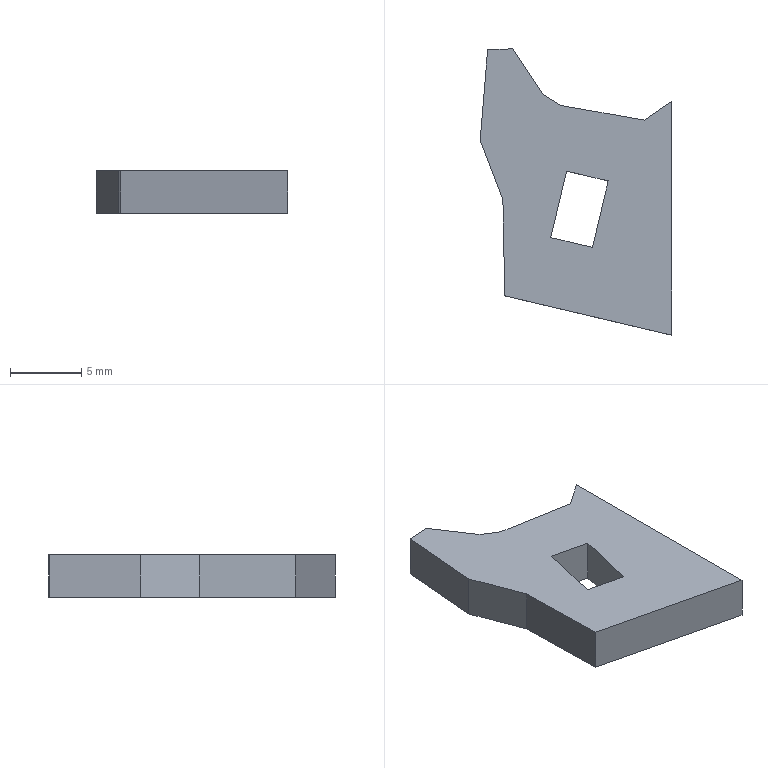Part | SolidWorks | features BaseBody 1 | 1 solid | 16 faces | box 13.422 x 20.055 x 3 mm | volume 525.703 mm3 | spline 9 | plane 7
STEP:
#1=CARTESIAN_POINT('',(-7.64,4.495,-1.5));
#2=VERTEX_POINT('',#1);
#3=CARTESIAN_POINT('',(-8.743,-0.1604,-1.5));
#4=VERTEX_POINT('',#3);
#5=CARTESIAN_POINT('',(-8.242,1.953,-1.5));
#6=DIRECTION('',(-0.2306,-0.9731,0.));
#7=VECTOR('',#6,1000.);
#8=LINE('',#5,#7);
#9=EDGE_CURVE('',#2,#4,#8,.T.);
#10=ORIENTED_EDGE('',*,*,#9,.F.);
#11=CARTESIAN_POINT('',(-7.64,4.495,1.5));
#12=VERTEX_POINT('',#11);
#13=CARTESIAN_POINT('',(-7.64,4.495,1.5));
#14=DIRECTION('',(0.,0.,-1.));
#15=VECTOR('',#14,1000.);
#16=LINE('',#13,#15);
#17=EDGE_CURVE('',#12,#2,#16,.T.);
#18=ORIENTED_EDGE('',*,*,#17,.F.);
#19=CARTESIAN_POINT('',(-8.743,-0.1604,1.5));
#20=VERTEX_POINT('',#19);
#21=CARTESIAN_POINT('',(-8.242,1.953,1.5));
#22=DIRECTION('',(-0.2306,-0.9731,0.));
#23=VECTOR('',#22,1000.);
#24=LINE('',#21,#23);
#25=EDGE_CURVE('',#12,#20,#24,.T.);
#26=ORIENTED_EDGE('',*,*,#25,.T.);
#27=CARTESIAN_POINT('',(-8.743,-0.1604,1.5));
#28=DIRECTION('',(0.,0.,-1.));
#29=VECTOR('',#28,1000.);
#30=LINE('',#27,#29);
#31=EDGE_CURVE('',#20,#4,#30,.T.);
#32=ORIENTED_EDGE('',*,*,#31,.T.);
#33=EDGE_LOOP('',(#10,#18,#26,#32));
#34=FACE_OUTER_BOUND('',#33,.T.);
#35=CARTESIAN_POINT('',(-8.242,1.953,1.5));
#36=DIRECTION('',(0.9731,-0.2306,0.));
#37=DIRECTION('',(0.,0.,-1.));
#38=AXIS2_PLACEMENT_3D('',#35,#36,#37);
#39=PLANE('',#38);
#40=ADVANCED_FACE('',(#34),#39,.T.);
#41=CARTESIAN_POINT('',(-4.721,3.803,-1.5));
#42=VERTEX_POINT('',#41);
#43=CARTESIAN_POINT('',(0.6024,2.542,-1.5));
#44=DIRECTION('',(-0.9731,0.2306,0.));
#45=VECTOR('',#44,1000.);
#46=LINE('',#43,#45);
#47=EDGE_CURVE('',#42,#2,#46,.T.);
#48=ORIENTED_EDGE('',*,*,#47,.F.);
#49=CARTESIAN_POINT('',(-4.721,3.803,1.5));
#50=VERTEX_POINT('',#49);
#51=CARTESIAN_POINT('',(-4.721,3.803,1.5));
#52=DIRECTION('',(0.,0.,-1.));
#53=VECTOR('',#52,1000.);
#54=LINE('',#51,#53);
#55=EDGE_CURVE('',#50,#42,#54,.T.);
#56=ORIENTED_EDGE('',*,*,#55,.F.);
#57=CARTESIAN_POINT('',(0.6024,2.542,1.5));
#58=DIRECTION('',(-0.9731,0.2306,0.));
#59=VECTOR('',#58,1000.);
#60=LINE('',#57,#59);
#61=EDGE_CURVE('',#50,#12,#60,.T.);
#62=ORIENTED_EDGE('',*,*,#61,.T.);
#63=ORIENTED_EDGE('',*,*,#17,.T.);
#64=EDGE_LOOP('',(#48,#56,#62,#63));
#65=FACE_OUTER_BOUND('',#64,.T.);
#66=CARTESIAN_POINT('',(0.6024,2.542,1.5));
#67=DIRECTION('',(-0.2306,-0.9731,0.));
#68=DIRECTION('',(-0.9731,0.2306,0.));
#69=AXIS2_PLACEMENT_3D('',#66,#67,#68);
#70=PLANE('',#69);
#71=ADVANCED_FACE('',(#65),#70,.T.);
#72=CARTESIAN_POINT('',(-5.824,-0.8521,-1.5));
#73=VERTEX_POINT('',#72);
#74=CARTESIAN_POINT('',(-5.323,1.261,-1.5));
#75=DIRECTION('',(-0.2306,-0.9731,0.));
#76=VECTOR('',#75,1000.);
#77=LINE('',#74,#76);
#78=EDGE_CURVE('',#42,#73,#77,.T.);
#79=ORIENTED_EDGE('',*,*,#78,.T.);
#80=CARTESIAN_POINT('',(-5.824,-0.8521,1.5));
#81=VERTEX_POINT('',#80);
#82=CARTESIAN_POINT('',(-5.824,-0.8521,1.5));
#83=DIRECTION('',(0.,0.,-1.));
#84=VECTOR('',#83,1000.);
#85=LINE('',#82,#84);
#86=EDGE_CURVE('',#81,#73,#85,.T.);
#87=ORIENTED_EDGE('',*,*,#86,.F.);
#88=CARTESIAN_POINT('',(-5.323,1.261,1.5));
#89=DIRECTION('',(-0.2306,-0.9731,0.));
#90=VECTOR('',#89,1000.);
#91=LINE('',#88,#90);
#92=EDGE_CURVE('',#50,#81,#91,.T.);
#93=ORIENTED_EDGE('',*,*,#92,.F.);
#94=ORIENTED_EDGE('',*,*,#55,.T.);
#95=EDGE_LOOP('',(#79,#87,#93,#94));
#96=FACE_OUTER_BOUND('',#95,.T.);
#97=CARTESIAN_POINT('',(-5.323,1.261,1.5));
#98=DIRECTION('',(0.9731,-0.2306,0.));
#99=DIRECTION('',(0.,0.,-1.));
#100=AXIS2_PLACEMENT_3D('',#97,#98,#99);
#101=PLANE('',#100);
#102=ADVANCED_FACE('',(#96),#101,.F.);
#103=CARTESIAN_POINT('',(-0.5008,-2.113,-1.5));
#104=DIRECTION('',(-0.9731,0.2306,0.));
#105=VECTOR('',#104,1000.);
#106=LINE('',#103,#105);
#107=EDGE_CURVE('',#73,#4,#106,.T.);
#108=ORIENTED_EDGE('',*,*,#107,.T.);
#109=ORIENTED_EDGE('',*,*,#31,.F.);
#110=CARTESIAN_POINT('',(-0.5008,-2.113,1.5));
#111=DIRECTION('',(-0.9731,0.2306,0.));
#112=VECTOR('',#111,1000.);
#113=LINE('',#110,#112);
#114=EDGE_CURVE('',#81,#20,#113,.T.);
#115=ORIENTED_EDGE('',*,*,#114,.F.);
#116=ORIENTED_EDGE('',*,*,#86,.T.);
#117=EDGE_LOOP('',(#108,#109,#115,#116));
#118=FACE_OUTER_BOUND('',#117,.T.);
#119=CARTESIAN_POINT('',(-0.5008,-2.113,1.5));
#120=DIRECTION('',(-0.2306,-0.9731,0.));
#121=DIRECTION('',(-0.9731,0.2306,0.));
#122=AXIS2_PLACEMENT_3D('',#119,#120,#121);
#123=PLANE('',#122);
#124=ADVANCED_FACE('',(#118),#123,.F.);
#125=ORIENTED_EDGE('',*,*,#9,.T.);
#126=ORIENTED_EDGE('',*,*,#107,.F.);
#127=ORIENTED_EDGE('',*,*,#78,.F.);
#128=ORIENTED_EDGE('',*,*,#47,.T.);
#129=EDGE_LOOP('',(#125,#126,#127,#128));
#130=FACE_BOUND('',#129,.T.);
#131=CARTESIAN_POINT('',(-0.264,9.379,-1.5));
#132=VERTEX_POINT('',#131);
#133=CARTESIAN_POINT('',(-2.191,8.063,-1.5));
#134=VERTEX_POINT('',#133);
#135=CARTESIAN_POINT('',(-0.264,9.379,-1.5));
#136=CARTESIAN_POINT('',(-0.9053,8.941,-1.5));
#137=CARTESIAN_POINT('',(-1.55,8.503,-1.5));
#138=CARTESIAN_POINT('',(-2.191,8.063,-1.5));
#139=B_SPLINE_CURVE_WITH_KNOTS('',3,(#135,#136,#137,#138),.UNSPECIFIED.,.F.,.F.,(4,4),(0.4737,0.5263),.UNSPECIFIED.);
#140=EDGE_CURVE('',#132,#134,#139,.T.);
#141=ORIENTED_EDGE('',*,*,#140,.F.);
#142=CARTESIAN_POINT('',(-0.264,-6.995,-1.5));
#143=VERTEX_POINT('',#142);
#144=CARTESIAN_POINT('',(-0.264,9.379,-1.5));
#145=DIRECTION('',(0.,-1.,0.));
#146=VECTOR('',#145,1000.);
#147=LINE('',#144,#146);
#148=EDGE_CURVE('',#132,#143,#147,.T.);
#149=ORIENTED_EDGE('',*,*,#148,.T.);
#150=CARTESIAN_POINT('',(-11.964,-4.235,-1.5));
#151=VERTEX_POINT('',#150);
#152=CARTESIAN_POINT('',(-11.964,-4.235,-1.5));
#153=CARTESIAN_POINT('',(-8.063,-5.155,-1.5));
#154=CARTESIAN_POINT('',(-4.164,-6.075,-1.5));
#155=CARTESIAN_POINT('',(-0.264,-6.995,-1.5));
#156=B_SPLINE_CURVE_WITH_KNOTS('',3,(#152,#153,#154,#155),.UNSPECIFIED.,.F.,.F.,(4,4),(0.8947,1.),.UNSPECIFIED.);
#157=EDGE_CURVE('',#151,#143,#156,.T.);
#158=ORIENTED_EDGE('',*,*,#157,.F.);
#159=CARTESIAN_POINT('',(-12.094,2.485,-1.5));
#160=VERTEX_POINT('',#159);
#161=CARTESIAN_POINT('',(-12.094,2.485,-1.5));
#162=CARTESIAN_POINT('',(-12.051,0.2468,-1.5));
#163=CARTESIAN_POINT('',(-12.008,-1.995,-1.5));
#164=CARTESIAN_POINT('',(-11.964,-4.235,-1.5));
#165=B_SPLINE_CURVE_WITH_KNOTS('',3,(#161,#162,#163,#164),.UNSPECIFIED.,.F.,.F.,(4,4),(0.8421,0.8947),.UNSPECIFIED.);
#166=EDGE_CURVE('',#160,#151,#165,.T.);
#167=ORIENTED_EDGE('',*,*,#166,.F.);
#168=CARTESIAN_POINT('',(-13.686,6.633,-1.5));
#169=VERTEX_POINT('',#168);
#170=CARTESIAN_POINT('',(-13.686,6.633,-1.5));
#171=CARTESIAN_POINT('',(-13.157,5.251,-1.5));
#172=CARTESIAN_POINT('',(-12.626,3.868,-1.5));
#173=CARTESIAN_POINT('',(-12.094,2.485,-1.5));
#174=B_SPLINE_CURVE_WITH_KNOTS('',3,(#170,#171,#172,#173),.UNSPECIFIED.,.F.,.F.,(4,4),(0.7895,0.8421),.UNSPECIFIED.);
#175=EDGE_CURVE('',#169,#160,#174,.T.);
#176=ORIENTED_EDGE('',*,*,#175,.F.);
#177=CARTESIAN_POINT('',(-13.167,12.98,-1.5));
#178=VERTEX_POINT('',#177);
#179=CARTESIAN_POINT('',(-13.167,12.98,-1.5));
#180=CARTESIAN_POINT('',(-13.338,10.864,-1.5));
#181=CARTESIAN_POINT('',(-13.513,8.749,-1.5));
#182=CARTESIAN_POINT('',(-13.686,6.633,-1.5));
#183=B_SPLINE_CURVE_WITH_KNOTS('',3,(#179,#180,#181,#182),.UNSPECIFIED.,.F.,.F.,(4,4),(0.7368,0.7895),.UNSPECIFIED.);
#184=EDGE_CURVE('',#178,#169,#183,.T.);
#185=ORIENTED_EDGE('',*,*,#184,.F.);
#186=CARTESIAN_POINT('',(-11.425,13.059,-1.5));
#187=VERTEX_POINT('',#186);
#188=CARTESIAN_POINT('',(-11.425,13.059,-1.5));
#189=CARTESIAN_POINT('',(-12.004,13.035,-1.5));
#190=CARTESIAN_POINT('',(-12.584,13.006,-1.5));
#191=CARTESIAN_POINT('',(-13.167,12.98,-1.5));
#192=B_SPLINE_CURVE_WITH_KNOTS('',3,(#188,#189,#190,#191),.UNSPECIFIED.,.F.,.F.,(4,4),(0.6842,0.7368),.UNSPECIFIED.);
#193=EDGE_CURVE('',#187,#178,#192,.T.);
#194=ORIENTED_EDGE('',*,*,#193,.F.);
#195=CARTESIAN_POINT('',(-9.322,9.892,-1.5));
#196=VERTEX_POINT('',#195);
#197=CARTESIAN_POINT('',(-9.322,9.892,-1.5));
#198=CARTESIAN_POINT('',(-10.022,10.947,-1.5));
#199=CARTESIAN_POINT('',(-10.724,12.004,-1.5));
#200=CARTESIAN_POINT('',(-11.425,13.059,-1.5));
#201=B_SPLINE_CURVE_WITH_KNOTS('',3,(#197,#198,#199,#200),.UNSPECIFIED.,.F.,.F.,(4,4),(0.6316,0.6842),.UNSPECIFIED.);
#202=EDGE_CURVE('',#196,#187,#201,.T.);
#203=ORIENTED_EDGE('',*,*,#202,.F.);
#204=CARTESIAN_POINT('',(-8.049,9.09,-1.5));
#205=VERTEX_POINT('',#204);
#206=CARTESIAN_POINT('',(-8.049,9.09,-1.5));
#207=CARTESIAN_POINT('',(-8.471,9.357,-1.5));
#208=CARTESIAN_POINT('',(-8.897,9.624,-1.5));
#209=CARTESIAN_POINT('',(-9.322,9.892,-1.5));
#210=B_SPLINE_CURVE_WITH_KNOTS('',3,(#206,#207,#208,#209),.UNSPECIFIED.,.F.,.F.,(4,4),(0.5789,0.6316),.UNSPECIFIED.);
#211=EDGE_CURVE('',#205,#196,#210,.T.);
#212=ORIENTED_EDGE('',*,*,#211,.F.);
#213=CARTESIAN_POINT('',(-2.191,8.063,-1.5));
#214=CARTESIAN_POINT('',(-4.141,8.406,-1.5));
#215=CARTESIAN_POINT('',(-6.094,8.747,-1.5));
#216=CARTESIAN_POINT('',(-8.049,9.09,-1.5));
#217=B_SPLINE_CURVE_WITH_KNOTS('',3,(#213,#214,#215,#216),.UNSPECIFIED.,.F.,.F.,(4,4),(0.5263,0.5789),.UNSPECIFIED.);
#218=EDGE_CURVE('',#134,#205,#217,.T.);
#219=ORIENTED_EDGE('',*,*,#218,.F.);
#220=EDGE_LOOP('',(#141,#149,#158,#167,#176,#185,#194,#203,#212,#219));
#221=FACE_OUTER_BOUND('',#220,.T.);
#222=CARTESIAN_POINT('',(-1.228,8.722,-1.5));
#223=DIRECTION('',(0.,0.,1.));
#224=DIRECTION('',(1.,0.,0.));
#225=AXIS2_PLACEMENT_3D('',#222,#223,#224);
#226=PLANE('',#225);
#227=ADVANCED_FACE('',(#130,#221),#226,.F.);
#228=ORIENTED_EDGE('',*,*,#114,.T.);
#229=ORIENTED_EDGE('',*,*,#25,.F.);
#230=ORIENTED_EDGE('',*,*,#61,.F.);
#231=ORIENTED_EDGE('',*,*,#92,.T.);
#232=EDGE_LOOP('',(#228,#229,#230,#231));
#233=FACE_BOUND('',#232,.T.);
#234=CARTESIAN_POINT('',(-0.264,9.379,1.5));
#235=VERTEX_POINT('',#234);
#236=CARTESIAN_POINT('',(-2.191,8.063,1.5));
#237=VERTEX_POINT('',#236);
#238=CARTESIAN_POINT('',(-0.264,9.379,1.5));
#239=CARTESIAN_POINT('',(-0.9053,8.941,1.5));
#240=CARTESIAN_POINT('',(-1.55,8.503,1.5));
#241=CARTESIAN_POINT('',(-2.191,8.063,1.5));
#242=B_SPLINE_CURVE_WITH_KNOTS('',3,(#238,#239,#240,#241),.UNSPECIFIED.,.F.,.F.,(4,4),(0.4737,0.5263),.UNSPECIFIED.);
#243=EDGE_CURVE('',#235,#237,#242,.T.);
#244=ORIENTED_EDGE('',*,*,#243,.T.);
#245=CARTESIAN_POINT('',(-8.049,9.09,1.5));
#246=VERTEX_POINT('',#245);
#247=CARTESIAN_POINT('',(-2.191,8.063,1.5));
#248=CARTESIAN_POINT('',(-4.141,8.406,1.5));
#249=CARTESIAN_POINT('',(-6.094,8.747,1.5));
#250=CARTESIAN_POINT('',(-8.049,9.09,1.5));
#251=B_SPLINE_CURVE_WITH_KNOTS('',3,(#247,#248,#249,#250),.UNSPECIFIED.,.F.,.F.,(4,4),(0.5263,0.5789),.UNSPECIFIED.);
#252=EDGE_CURVE('',#237,#246,#251,.T.);
#253=ORIENTED_EDGE('',*,*,#252,.T.);
#254=CARTESIAN_POINT('',(-9.322,9.892,1.5));
#255=VERTEX_POINT('',#254);
#256=CARTESIAN_POINT('',(-8.049,9.09,1.5));
#257=CARTESIAN_POINT('',(-8.471,9.357,1.5));
#258=CARTESIAN_POINT('',(-8.897,9.624,1.5));
#259=CARTESIAN_POINT('',(-9.322,9.892,1.5));
#260=B_SPLINE_CURVE_WITH_KNOTS('',3,(#256,#257,#258,#259),.UNSPECIFIED.,.F.,.F.,(4,4),(0.5789,0.6316),.UNSPECIFIED.);
#261=EDGE_CURVE('',#246,#255,#260,.T.);
#262=ORIENTED_EDGE('',*,*,#261,.T.);
#263=CARTESIAN_POINT('',(-11.425,13.059,1.5));
#264=VERTEX_POINT('',#263);
#265=CARTESIAN_POINT('',(-9.322,9.892,1.5));
#266=CARTESIAN_POINT('',(-10.022,10.947,1.5));
#267=CARTESIAN_POINT('',(-10.724,12.004,1.5));
#268=CARTESIAN_POINT('',(-11.425,13.059,1.5));
#269=B_SPLINE_CURVE_WITH_KNOTS('',3,(#265,#266,#267,#268),.UNSPECIFIED.,.F.,.F.,(4,4),(0.6316,0.6842),.UNSPECIFIED.);
#270=EDGE_CURVE('',#255,#264,#269,.T.);
#271=ORIENTED_EDGE('',*,*,#270,.T.);
#272=CARTESIAN_POINT('',(-13.167,12.98,1.5));
#273=VERTEX_POINT('',#272);
#274=CARTESIAN_POINT('',(-11.425,13.059,1.5));
#275=CARTESIAN_POINT('',(-12.004,13.035,1.5));
#276=CARTESIAN_POINT('',(-12.584,13.006,1.5));
#277=CARTESIAN_POINT('',(-13.167,12.98,1.5));
#278=B_SPLINE_CURVE_WITH_KNOTS('',3,(#274,#275,#276,#277),.UNSPECIFIED.,.F.,.F.,(4,4),(0.6842,0.7368),.UNSPECIFIED.);
#279=EDGE_CURVE('',#264,#273,#278,.T.);
#280=ORIENTED_EDGE('',*,*,#279,.T.);
#281=CARTESIAN_POINT('',(-13.686,6.633,1.5));
#282=VERTEX_POINT('',#281);
#283=CARTESIAN_POINT('',(-13.167,12.98,1.5));
#284=CARTESIAN_POINT('',(-13.338,10.864,1.5));
#285=CARTESIAN_POINT('',(-13.513,8.749,1.5));
#286=CARTESIAN_POINT('',(-13.686,6.633,1.5));
#287=B_SPLINE_CURVE_WITH_KNOTS('',3,(#283,#284,#285,#286),.UNSPECIFIED.,.F.,.F.,(4,4),(0.7368,0.7895),.UNSPECIFIED.);
#288=EDGE_CURVE('',#273,#282,#287,.T.);
#289=ORIENTED_EDGE('',*,*,#288,.T.);
#290=CARTESIAN_POINT('',(-12.094,2.485,1.5));
#291=VERTEX_POINT('',#290);
#292=CARTESIAN_POINT('',(-13.686,6.633,1.5));
#293=CARTESIAN_POINT('',(-13.157,5.251,1.5));
#294=CARTESIAN_POINT('',(-12.626,3.868,1.5));
#295=CARTESIAN_POINT('',(-12.094,2.485,1.5));
#296=B_SPLINE_CURVE_WITH_KNOTS('',3,(#292,#293,#294,#295),.UNSPECIFIED.,.F.,.F.,(4,4),(0.7895,0.8421),.UNSPECIFIED.);
#297=EDGE_CURVE('',#282,#291,#296,.T.);
#298=ORIENTED_EDGE('',*,*,#297,.T.);
#299=CARTESIAN_POINT('',(-11.964,-4.235,1.5));
#300=VERTEX_POINT('',#299);
#301=CARTESIAN_POINT('',(-12.094,2.485,1.5));
#302=CARTESIAN_POINT('',(-12.051,0.2468,1.5));
#303=CARTESIAN_POINT('',(-12.008,-1.995,1.5));
#304=CARTESIAN_POINT('',(-11.964,-4.235,1.5));
#305=B_SPLINE_CURVE_WITH_KNOTS('',3,(#301,#302,#303,#304),.UNSPECIFIED.,.F.,.F.,(4,4),(0.8421,0.8947),.UNSPECIFIED.);
#306=EDGE_CURVE('',#291,#300,#305,.T.);
#307=ORIENTED_EDGE('',*,*,#306,.T.);
#308=CARTESIAN_POINT('',(-0.264,-6.995,1.5));
#309=VERTEX_POINT('',#308);
#310=CARTESIAN_POINT('',(-11.964,-4.235,1.5));
#311=CARTESIAN_POINT('',(-8.063,-5.155,1.5));
#312=CARTESIAN_POINT('',(-4.164,-6.075,1.5));
#313=CARTESIAN_POINT('',(-0.264,-6.995,1.5));
#314=B_SPLINE_CURVE_WITH_KNOTS('',3,(#310,#311,#312,#313),.UNSPECIFIED.,.F.,.F.,(4,4),(0.8947,1.),.UNSPECIFIED.);
#315=EDGE_CURVE('',#300,#309,#314,.T.);
#316=ORIENTED_EDGE('',*,*,#315,.T.);
#317=CARTESIAN_POINT('',(-0.264,9.379,1.5));
#318=DIRECTION('',(0.,-1.,0.));
#319=VECTOR('',#318,1000.);
#320=LINE('',#317,#319);
#321=EDGE_CURVE('',#235,#309,#320,.T.);
#322=ORIENTED_EDGE('',*,*,#321,.F.);
#323=EDGE_LOOP('',(#244,#253,#262,#271,#280,#289,#298,#307,#316,#322));
#324=FACE_OUTER_BOUND('',#323,.T.);
#325=CARTESIAN_POINT('',(-1.228,8.722,1.5));
#326=DIRECTION('',(0.,0.,1.));
#327=DIRECTION('',(1.,0.,0.));
#328=AXIS2_PLACEMENT_3D('',#325,#326,#327);
#329=PLANE('',#328);
#330=ADVANCED_FACE('',(#233,#324),#329,.T.);
#331=ORIENTED_EDGE('',*,*,#148,.F.);
#332=CARTESIAN_POINT('',(-0.264,9.379,1.5));
#333=DIRECTION('',(0.,0.,-1.));
#334=VECTOR('',#333,1000.);
#335=LINE('',#332,#334);
#336=EDGE_CURVE('',#235,#132,#335,.T.);
#337=ORIENTED_EDGE('',*,*,#336,.F.);
#338=ORIENTED_EDGE('',*,*,#321,.T.);
#339=CARTESIAN_POINT('',(-0.264,-6.995,1.5));
#340=DIRECTION('',(0.,0.,-1.));
#341=VECTOR('',#340,1000.);
#342=LINE('',#339,#341);
#343=EDGE_CURVE('',#309,#143,#342,.T.);
#344=ORIENTED_EDGE('',*,*,#343,.T.);
#345=EDGE_LOOP('',(#331,#337,#338,#344));
#346=FACE_OUTER_BOUND('',#345,.T.);
#347=CARTESIAN_POINT('',(-0.264,9.379,1.5));
#348=DIRECTION('',(1.,0.,0.));
#349=DIRECTION('',(0.,1.,0.));
#350=AXIS2_PLACEMENT_3D('',#347,#348,#349);
#351=PLANE('',#350);
#352=ADVANCED_FACE('',(#346),#351,.T.);
#353=ORIENTED_EDGE('',*,*,#157,.T.);
#354=ORIENTED_EDGE('',*,*,#343,.F.);
#355=ORIENTED_EDGE('',*,*,#315,.F.);
#356=CARTESIAN_POINT('',(-11.964,-4.235,1.5));
#357=DIRECTION('',(0.,0.,-1.));
#358=VECTOR('',#357,1000.);
#359=LINE('',#356,#358);
#360=EDGE_CURVE('',#300,#151,#359,.T.);
#361=ORIENTED_EDGE('',*,*,#360,.T.);
#362=EDGE_LOOP('',(#353,#354,#355,#361));
#363=FACE_OUTER_BOUND('',#362,.T.);
#364=CARTESIAN_POINT('',(-11.964,-4.235,1.5));
#365=CARTESIAN_POINT('',(-11.964,-4.235,-1.5));
#366=CARTESIAN_POINT('',(-8.063,-5.155,1.5));
#367=CARTESIAN_POINT('',(-8.063,-5.155,-1.5));
#368=CARTESIAN_POINT('',(-4.164,-6.075,1.5));
#369=CARTESIAN_POINT('',(-4.164,-6.075,-1.5));
#370=CARTESIAN_POINT('',(-0.264,-6.995,1.5));
#371=CARTESIAN_POINT('',(-0.264,-6.995,-1.5));
#372=B_SPLINE_SURFACE_WITH_KNOTS('',3,1,((#364,#365),(#366,#367),(#368,#369),(#370,#371)),.UNSPECIFIED.,.F.,.F.,.F.,(4,4),(2,2),(0.8947,1.),(0.,1.),.UNSPECIFIED.);
#373=ADVANCED_FACE('',(#363),#372,.F.);
#374=ORIENTED_EDGE('',*,*,#166,.T.);
#375=ORIENTED_EDGE('',*,*,#360,.F.);
#376=ORIENTED_EDGE('',*,*,#306,.F.);
#377=CARTESIAN_POINT('',(-12.094,2.485,1.5));
#378=DIRECTION('',(0.,0.,-1.));
#379=VECTOR('',#378,1000.);
#380=LINE('',#377,#379);
#381=EDGE_CURVE('',#291,#160,#380,.T.);
#382=ORIENTED_EDGE('',*,*,#381,.T.);
#383=EDGE_LOOP('',(#374,#375,#376,#382));
#384=FACE_OUTER_BOUND('',#383,.T.);
#385=CARTESIAN_POINT('',(-12.094,2.485,1.5));
#386=CARTESIAN_POINT('',(-12.094,2.485,-1.5));
#387=CARTESIAN_POINT('',(-12.051,0.2468,1.5));
#388=CARTESIAN_POINT('',(-12.051,0.2468,-1.5));
#389=CARTESIAN_POINT('',(-12.008,-1.995,1.5));
#390=CARTESIAN_POINT('',(-12.008,-1.995,-1.5));
#391=CARTESIAN_POINT('',(-11.964,-4.235,1.5));
#392=CARTESIAN_POINT('',(-11.964,-4.235,-1.5));
#393=B_SPLINE_SURFACE_WITH_KNOTS('',3,1,((#385,#386),(#387,#388),(#389,#390),(#391,#392)),.UNSPECIFIED.,.F.,.F.,.F.,(4,4),(2,2),(0.8421,0.8947),(0.,1.),.UNSPECIFIED.);
#394=ADVANCED_FACE('',(#384),#393,.F.);
#395=ORIENTED_EDGE('',*,*,#175,.T.);
#396=ORIENTED_EDGE('',*,*,#381,.F.);
#397=ORIENTED_EDGE('',*,*,#297,.F.);
#398=CARTESIAN_POINT('',(-13.686,6.633,1.5));
#399=DIRECTION('',(0.,0.,-1.));
#400=VECTOR('',#399,1000.);
#401=LINE('',#398,#400);
#402=EDGE_CURVE('',#282,#169,#401,.T.);
#403=ORIENTED_EDGE('',*,*,#402,.T.);
#404=EDGE_LOOP('',(#395,#396,#397,#403));
#405=FACE_OUTER_BOUND('',#404,.T.);
#406=CARTESIAN_POINT('',(-13.686,6.633,1.5));
#407=CARTESIAN_POINT('',(-13.686,6.633,-1.5));
#408=CARTESIAN_POINT('',(-13.157,5.251,1.5));
#409=CARTESIAN_POINT('',(-13.157,5.251,-1.5));
#410=CARTESIAN_POINT('',(-12.626,3.868,1.5));
#411=CARTESIAN_POINT('',(-12.626,3.868,-1.5));
#412=CARTESIAN_POINT('',(-12.094,2.485,1.5));
#413=CARTESIAN_POINT('',(-12.094,2.485,-1.5));
#414=B_SPLINE_SURFACE_WITH_KNOTS('',3,1,((#406,#407),(#408,#409),(#410,#411),(#412,#413)),.UNSPECIFIED.,.F.,.F.,.F.,(4,4),(2,2),(0.7895,0.8421),(0.,1.),.UNSPECIFIED.);
#415=ADVANCED_FACE('',(#405),#414,.F.);
#416=ORIENTED_EDGE('',*,*,#184,.T.);
#417=ORIENTED_EDGE('',*,*,#402,.F.);
#418=ORIENTED_EDGE('',*,*,#288,.F.);
#419=CARTESIAN_POINT('',(-13.167,12.98,1.5));
#420=DIRECTION('',(0.,0.,-1.));
#421=VECTOR('',#420,1000.);
#422=LINE('',#419,#421);
#423=EDGE_CURVE('',#273,#178,#422,.T.);
#424=ORIENTED_EDGE('',*,*,#423,.T.);
#425=EDGE_LOOP('',(#416,#417,#418,#424));
#426=FACE_OUTER_BOUND('',#425,.T.);
#427=CARTESIAN_POINT('',(-13.167,12.98,1.5));
#428=CARTESIAN_POINT('',(-13.167,12.98,-1.5));
#429=CARTESIAN_POINT('',(-13.338,10.864,1.5));
#430=CARTESIAN_POINT('',(-13.338,10.864,-1.5));
#431=CARTESIAN_POINT('',(-13.513,8.749,1.5));
#432=CARTESIAN_POINT('',(-13.513,8.749,-1.5));
#433=CARTESIAN_POINT('',(-13.686,6.633,1.5));
#434=CARTESIAN_POINT('',(-13.686,6.633,-1.5));
#435=B_SPLINE_SURFACE_WITH_KNOTS('',3,1,((#427,#428),(#429,#430),(#431,#432),(#433,#434)),.UNSPECIFIED.,.F.,.F.,.F.,(4,4),(2,2),(0.7368,0.7895),(0.,1.),.UNSPECIFIED.);
#436=ADVANCED_FACE('',(#426),#435,.F.);
#437=ORIENTED_EDGE('',*,*,#193,.T.);
#438=ORIENTED_EDGE('',*,*,#423,.F.);
#439=ORIENTED_EDGE('',*,*,#279,.F.);
#440=CARTESIAN_POINT('',(-11.425,13.059,1.5));
#441=DIRECTION('',(0.,0.,-1.));
#442=VECTOR('',#441,1000.);
#443=LINE('',#440,#442);
#444=EDGE_CURVE('',#264,#187,#443,.T.);
#445=ORIENTED_EDGE('',*,*,#444,.T.);
#446=EDGE_LOOP('',(#437,#438,#439,#445));
#447=FACE_OUTER_BOUND('',#446,.T.);
#448=CARTESIAN_POINT('',(-11.425,13.059,1.5));
#449=CARTESIAN_POINT('',(-11.425,13.059,-1.5));
#450=CARTESIAN_POINT('',(-12.004,13.035,1.5));
#451=CARTESIAN_POINT('',(-12.004,13.035,-1.5));
#452=CARTESIAN_POINT('',(-12.584,13.006,1.5));
#453=CARTESIAN_POINT('',(-12.584,13.006,-1.5));
#454=CARTESIAN_POINT('',(-13.167,12.98,1.5));
#455=CARTESIAN_POINT('',(-13.167,12.98,-1.5));
#456=B_SPLINE_SURFACE_WITH_KNOTS('',3,1,((#448,#449),(#450,#451),(#452,#453),(#454,#455)),.UNSPECIFIED.,.F.,.F.,.F.,(4,4),(2,2),(0.6842,0.7368),(0.,1.),.UNSPECIFIED.);
#457=ADVANCED_FACE('',(#447),#456,.F.);
#458=ORIENTED_EDGE('',*,*,#202,.T.);
#459=ORIENTED_EDGE('',*,*,#444,.F.);
#460=ORIENTED_EDGE('',*,*,#270,.F.);
#461=CARTESIAN_POINT('',(-9.322,9.892,1.5));
#462=DIRECTION('',(0.,0.,-1.));
#463=VECTOR('',#462,1000.);
#464=LINE('',#461,#463);
#465=EDGE_CURVE('',#255,#196,#464,.T.);
#466=ORIENTED_EDGE('',*,*,#465,.T.);
#467=EDGE_LOOP('',(#458,#459,#460,#466));
#468=FACE_OUTER_BOUND('',#467,.T.);
#469=CARTESIAN_POINT('',(-9.322,9.892,1.5));
#470=CARTESIAN_POINT('',(-9.322,9.892,-1.5));
#471=CARTESIAN_POINT('',(-10.022,10.947,1.5));
#472=CARTESIAN_POINT('',(-10.022,10.947,-1.5));
#473=CARTESIAN_POINT('',(-10.724,12.004,1.5));
#474=CARTESIAN_POINT('',(-10.724,12.004,-1.5));
#475=CARTESIAN_POINT('',(-11.425,13.059,1.5));
#476=CARTESIAN_POINT('',(-11.425,13.059,-1.5));
#477=B_SPLINE_SURFACE_WITH_KNOTS('',3,1,((#469,#470),(#471,#472),(#473,#474),(#475,#476)),.UNSPECIFIED.,.F.,.F.,.F.,(4,4),(2,2),(0.6316,0.6842),(0.,1.),.UNSPECIFIED.);
#478=ADVANCED_FACE('',(#468),#477,.F.);
#479=ORIENTED_EDGE('',*,*,#211,.T.);
#480=ORIENTED_EDGE('',*,*,#465,.F.);
#481=ORIENTED_EDGE('',*,*,#261,.F.);
#482=CARTESIAN_POINT('',(-8.049,9.09,1.5));
#483=DIRECTION('',(0.,0.,-1.));
#484=VECTOR('',#483,1000.);
#485=LINE('',#482,#484);
#486=EDGE_CURVE('',#246,#205,#485,.T.);
#487=ORIENTED_EDGE('',*,*,#486,.T.);
#488=EDGE_LOOP('',(#479,#480,#481,#487));
#489=FACE_OUTER_BOUND('',#488,.T.);
#490=CARTESIAN_POINT('',(-8.049,9.09,1.5));
#491=CARTESIAN_POINT('',(-8.049,9.09,-1.5));
#492=CARTESIAN_POINT('',(-8.471,9.357,1.5));
#493=CARTESIAN_POINT('',(-8.471,9.357,-1.5));
#494=CARTESIAN_POINT('',(-8.897,9.624,1.5));
#495=CARTESIAN_POINT('',(-8.897,9.624,-1.5));
#496=CARTESIAN_POINT('',(-9.322,9.892,1.5));
#497=CARTESIAN_POINT('',(-9.322,9.892,-1.5));
#498=B_SPLINE_SURFACE_WITH_KNOTS('',3,1,((#490,#491),(#492,#493),(#494,#495),(#496,#497)),.UNSPECIFIED.,.F.,.F.,.F.,(4,4),(2,2),(0.5789,0.6316),(0.,1.),.UNSPECIFIED.);
#499=ADVANCED_FACE('',(#489),#498,.F.);
#500=ORIENTED_EDGE('',*,*,#218,.T.);
#501=ORIENTED_EDGE('',*,*,#486,.F.);
#502=ORIENTED_EDGE('',*,*,#252,.F.);
#503=CARTESIAN_POINT('',(-2.191,8.063,1.5));
#504=DIRECTION('',(0.,0.,-1.));
#505=VECTOR('',#504,1000.);
#506=LINE('',#503,#505);
#507=EDGE_CURVE('',#237,#134,#506,.T.);
#508=ORIENTED_EDGE('',*,*,#507,.T.);
#509=EDGE_LOOP('',(#500,#501,#502,#508));
#510=FACE_OUTER_BOUND('',#509,.T.);
#511=CARTESIAN_POINT('',(-2.191,8.063,1.5));
#512=CARTESIAN_POINT('',(-2.191,8.063,-1.5));
#513=CARTESIAN_POINT('',(-4.141,8.406,1.5));
#514=CARTESIAN_POINT('',(-4.141,8.406,-1.5));
#515=CARTESIAN_POINT('',(-6.094,8.747,1.5));
#516=CARTESIAN_POINT('',(-6.094,8.747,-1.5));
#517=CARTESIAN_POINT('',(-8.049,9.09,1.5));
#518=CARTESIAN_POINT('',(-8.049,9.09,-1.5));
#519=B_SPLINE_SURFACE_WITH_KNOTS('',3,1,((#511,#512),(#513,#514),(#515,#516),(#517,#518)),.UNSPECIFIED.,.F.,.F.,.F.,(4,4),(2,2),(0.5263,0.5789),(0.,1.),.UNSPECIFIED.);
#520=ADVANCED_FACE('',(#510),#519,.F.);
#521=ORIENTED_EDGE('',*,*,#140,.T.);
#522=ORIENTED_EDGE('',*,*,#507,.F.);
#523=ORIENTED_EDGE('',*,*,#243,.F.);
#524=ORIENTED_EDGE('',*,*,#336,.T.);
#525=EDGE_LOOP('',(#521,#522,#523,#524));
#526=FACE_OUTER_BOUND('',#525,.T.);
#527=CARTESIAN_POINT('',(-0.264,9.379,1.5));
#528=CARTESIAN_POINT('',(-0.264,9.379,-1.5));
#529=CARTESIAN_POINT('',(-0.9053,8.941,1.5));
#530=CARTESIAN_POINT('',(-0.9053,8.941,-1.5));
#531=CARTESIAN_POINT('',(-1.55,8.503,1.5));
#532=CARTESIAN_POINT('',(-1.55,8.503,-1.5));
#533=CARTESIAN_POINT('',(-2.191,8.063,1.5));
#534=CARTESIAN_POINT('',(-2.191,8.063,-1.5));
#535=B_SPLINE_SURFACE_WITH_KNOTS('',3,1,((#527,#528),(#529,#530),(#531,#532),(#533,#534)),.UNSPECIFIED.,.F.,.F.,.F.,(4,4),(2,2),(0.4737,0.5263),(0.,1.),.UNSPECIFIED.);
#536=ADVANCED_FACE('',(#526),#535,.F.);
#537=CLOSED_SHELL('',(#40,#71,#102,#124,#227,#330,#352,#373,#394,#415,#436,#457,#478,#499,#520,#536));
#538=MANIFOLD_SOLID_BREP('',#537);
#539=CARTESIAN_POINT('',(0.,0.,0.));
#540=DIRECTION('',(0.,0.,1.));
#541=DIRECTION('',(1.,0.,0.));
#542=AXIS2_PLACEMENT_3D('',#539,#540,#541);
#543=(LENGTH_UNIT()NAMED_UNIT(*)SI_UNIT(.MILLI.,.METRE.));
#544=UNCERTAINTY_MEASURE_WITH_UNIT(LENGTH_MEASURE(0.00001),#543,'','');
#545=(NAMED_UNIT(*)PLANE_ANGLE_UNIT()SI_UNIT($,.RADIAN.));
#546=(NAMED_UNIT(*)SI_UNIT($,.STERADIAN.)SOLID_ANGLE_UNIT());
#547=(GEOMETRIC_REPRESENTATION_CONTEXT(3)GLOBAL_UNCERTAINTY_ASSIGNED_CONTEXT((#544))GLOBAL_UNIT_ASSIGNED_CONTEXT((#543,#545,#546))REPRESENTATION_CONTEXT('',''));
#548=ADVANCED_BREP_SHAPE_REPRESENTATION('',(#538,#542),#547);